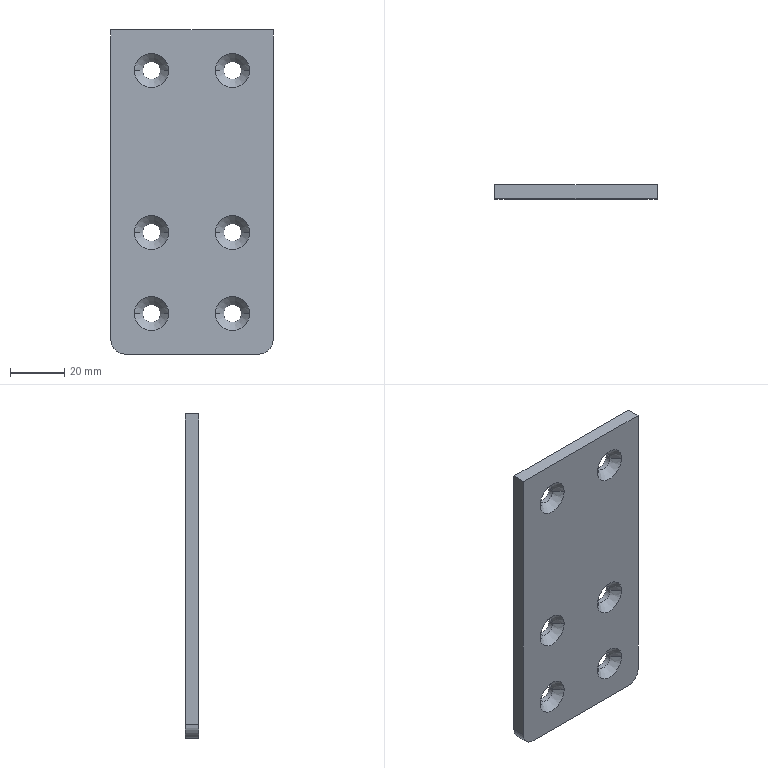Part | NX | features BREP 1 | 1 solid | 32 faces | box 60 x 5 x 120 mm | volume 34191 mm3 | cylinder 14 | cone 12 | plane 6 | commonest cylinder face diameters 6.6 x12 10 x2
STEP:
#1=CARTESIAN_POINT('',(-30.,0.,-70.));
#2=VERTEX_POINT('',#1);
#3=CARTESIAN_POINT('',(-30.,0.,45.));
#4=VERTEX_POINT('',#3);
#5=CARTESIAN_POINT('',(-30.,0.,-70.));
#6=DIRECTION('',(0.,0.,1.));
#7=VECTOR('',#6,1000.);
#8=LINE('',#5,#7);
#9=EDGE_CURVE('',#2,#4,#8,.T.);
#10=ORIENTED_EDGE('',*,*,#9,.F.);
#11=CARTESIAN_POINT('',(-25.,0.,-75.));
#12=VERTEX_POINT('',#11);
#13=CARTESIAN_POINT('',(-25.,0.,-70.));
#14=DIRECTION('',(0.,-1.,0.));
#15=DIRECTION('',(-1.,0.,0.));
#16=AXIS2_PLACEMENT_3D('',#13,#14,#15);
#17=CIRCLE('',#16,5.);
#18=EDGE_CURVE('',#2,#12,#17,.T.);
#19=ORIENTED_EDGE('',*,*,#18,.T.);
#20=CARTESIAN_POINT('',(25.,0.,-75.));
#21=VERTEX_POINT('',#20);
#22=CARTESIAN_POINT('',(25.,0.,-75.));
#23=DIRECTION('',(-1.,0.,0.));
#24=VECTOR('',#23,1000.);
#25=LINE('',#22,#24);
#26=EDGE_CURVE('',#21,#12,#25,.T.);
#27=ORIENTED_EDGE('',*,*,#26,.F.);
#28=CARTESIAN_POINT('',(30.,0.,-70.));
#29=VERTEX_POINT('',#28);
#30=CARTESIAN_POINT('',(25.,0.,-70.));
#31=DIRECTION('',(0.,-1.,0.));
#32=DIRECTION('',(0.,0.,-1.));
#33=AXIS2_PLACEMENT_3D('',#30,#31,#32);
#34=CIRCLE('',#33,5.);
#35=EDGE_CURVE('',#21,#29,#34,.T.);
#36=ORIENTED_EDGE('',*,*,#35,.T.);
#37=CARTESIAN_POINT('',(30.,0.,45.));
#38=VERTEX_POINT('',#37);
#39=CARTESIAN_POINT('',(30.,0.,45.));
#40=DIRECTION('',(0.,0.,-1.));
#41=VECTOR('',#40,1000.);
#42=LINE('',#39,#41);
#43=EDGE_CURVE('',#38,#29,#42,.T.);
#44=ORIENTED_EDGE('',*,*,#43,.F.);
#45=CARTESIAN_POINT('',(-30.,0.,45.));
#46=DIRECTION('',(1.,0.,0.));
#47=VECTOR('',#46,1000.);
#48=LINE('',#45,#47);
#49=EDGE_CURVE('',#4,#38,#48,.T.);
#50=ORIENTED_EDGE('',*,*,#49,.F.);
#51=EDGE_LOOP('',(#10,#19,#27,#36,#44,#50));
#52=FACE_BOUND('',#51,.T.);
#53=CARTESIAN_POINT('',(-8.7,0.,-60.));
#54=VERTEX_POINT('',#53);
#55=CARTESIAN_POINT('',(-21.3,0.,-60.));
#56=VERTEX_POINT('',#55);
#57=CARTESIAN_POINT('',(-15.,0.,-60.));
#58=DIRECTION('',(0.,-1.,0.));
#59=DIRECTION('',(1.,0.,0.));
#60=AXIS2_PLACEMENT_3D('',#57,#58,#59);
#61=CIRCLE('',#60,6.3);
#62=EDGE_CURVE('',#54,#56,#61,.T.);
#63=ORIENTED_EDGE('',*,*,#62,.F.);
#64=CARTESIAN_POINT('',(-15.,0.,-60.));
#65=DIRECTION('',(0.,-1.,0.));
#66=DIRECTION('',(-1.,0.,0.));
#67=AXIS2_PLACEMENT_3D('',#64,#65,#66);
#68=CIRCLE('',#67,6.3);
#69=EDGE_CURVE('',#56,#54,#68,.T.);
#70=ORIENTED_EDGE('',*,*,#69,.F.);
#71=EDGE_LOOP('',(#63,#70));
#72=FACE_BOUND('',#71,.T.);
#73=CARTESIAN_POINT('',(21.3,0.,-30.));
#74=VERTEX_POINT('',#73);
#75=CARTESIAN_POINT('',(8.7,0.,-30.));
#76=VERTEX_POINT('',#75);
#77=CARTESIAN_POINT('',(15.,0.,-30.));
#78=DIRECTION('',(0.,-1.,0.));
#79=DIRECTION('',(1.,0.,0.));
#80=AXIS2_PLACEMENT_3D('',#77,#78,#79);
#81=CIRCLE('',#80,6.3);
#82=EDGE_CURVE('',#74,#76,#81,.T.);
#83=ORIENTED_EDGE('',*,*,#82,.F.);
#84=CARTESIAN_POINT('',(15.,0.,-30.));
#85=DIRECTION('',(0.,-1.,0.));
#86=DIRECTION('',(-1.,0.,0.));
#87=AXIS2_PLACEMENT_3D('',#84,#85,#86);
#88=CIRCLE('',#87,6.3);
#89=EDGE_CURVE('',#76,#74,#88,.T.);
#90=ORIENTED_EDGE('',*,*,#89,.F.);
#91=EDGE_LOOP('',(#83,#90));
#92=FACE_BOUND('',#91,.T.);
#93=CARTESIAN_POINT('',(-8.7,0.,-30.));
#94=VERTEX_POINT('',#93);
#95=CARTESIAN_POINT('',(-21.3,0.,-30.));
#96=VERTEX_POINT('',#95);
#97=CARTESIAN_POINT('',(-15.,0.,-30.));
#98=DIRECTION('',(0.,-1.,0.));
#99=DIRECTION('',(1.,0.,0.));
#100=AXIS2_PLACEMENT_3D('',#97,#98,#99);
#101=CIRCLE('',#100,6.3);
#102=EDGE_CURVE('',#94,#96,#101,.T.);
#103=ORIENTED_EDGE('',*,*,#102,.F.);
#104=CARTESIAN_POINT('',(-15.,0.,-30.));
#105=DIRECTION('',(0.,-1.,0.));
#106=DIRECTION('',(-1.,0.,0.));
#107=AXIS2_PLACEMENT_3D('',#104,#105,#106);
#108=CIRCLE('',#107,6.3);
#109=EDGE_CURVE('',#96,#94,#108,.T.);
#110=ORIENTED_EDGE('',*,*,#109,.F.);
#111=EDGE_LOOP('',(#103,#110));
#112=FACE_BOUND('',#111,.T.);
#113=CARTESIAN_POINT('',(21.3,0.,30.));
#114=VERTEX_POINT('',#113);
#115=CARTESIAN_POINT('',(8.7,0.,30.));
#116=VERTEX_POINT('',#115);
#117=CARTESIAN_POINT('',(15.,0.,30.));
#118=DIRECTION('',(0.,1.,0.));
#119=DIRECTION('',(1.,0.,0.));
#120=AXIS2_PLACEMENT_3D('',#117,#118,#119);
#121=CIRCLE('',#120,6.3);
#122=EDGE_CURVE('',#114,#116,#121,.T.);
#123=ORIENTED_EDGE('',*,*,#122,.T.);
#124=CARTESIAN_POINT('',(15.,0.,30.));
#125=DIRECTION('',(0.,1.,0.));
#126=DIRECTION('',(-1.,0.,0.));
#127=AXIS2_PLACEMENT_3D('',#124,#125,#126);
#128=CIRCLE('',#127,6.3);
#129=EDGE_CURVE('',#116,#114,#128,.T.);
#130=ORIENTED_EDGE('',*,*,#129,.T.);
#131=EDGE_LOOP('',(#123,#130));
#132=FACE_BOUND('',#131,.T.);
#133=CARTESIAN_POINT('',(-8.7,0.,30.));
#134=VERTEX_POINT('',#133);
#135=CARTESIAN_POINT('',(-21.3,0.,30.));
#136=VERTEX_POINT('',#135);
#137=CARTESIAN_POINT('',(-15.,0.,30.));
#138=DIRECTION('',(0.,1.,0.));
#139=DIRECTION('',(1.,0.,0.));
#140=AXIS2_PLACEMENT_3D('',#137,#138,#139);
#141=CIRCLE('',#140,6.3);
#142=EDGE_CURVE('',#134,#136,#141,.T.);
#143=ORIENTED_EDGE('',*,*,#142,.T.);
#144=CARTESIAN_POINT('',(-15.,0.,30.));
#145=DIRECTION('',(0.,1.,0.));
#146=DIRECTION('',(-1.,0.,0.));
#147=AXIS2_PLACEMENT_3D('',#144,#145,#146);
#148=CIRCLE('',#147,6.3);
#149=EDGE_CURVE('',#136,#134,#148,.T.);
#150=ORIENTED_EDGE('',*,*,#149,.T.);
#151=EDGE_LOOP('',(#143,#150));
#152=FACE_BOUND('',#151,.T.);
#153=CARTESIAN_POINT('',(21.3,0.,-60.));
#154=VERTEX_POINT('',#153);
#155=CARTESIAN_POINT('',(8.7,0.,-60.));
#156=VERTEX_POINT('',#155);
#157=CARTESIAN_POINT('',(15.,0.,-60.));
#158=DIRECTION('',(0.,-1.,0.));
#159=DIRECTION('',(1.,0.,0.));
#160=AXIS2_PLACEMENT_3D('',#157,#158,#159);
#161=CIRCLE('',#160,6.3);
#162=EDGE_CURVE('',#154,#156,#161,.T.);
#163=ORIENTED_EDGE('',*,*,#162,.F.);
#164=CARTESIAN_POINT('',(15.,0.,-60.));
#165=DIRECTION('',(0.,-1.,0.));
#166=DIRECTION('',(-1.,0.,0.));
#167=AXIS2_PLACEMENT_3D('',#164,#165,#166);
#168=CIRCLE('',#167,6.3);
#169=EDGE_CURVE('',#156,#154,#168,.T.);
#170=ORIENTED_EDGE('',*,*,#169,.F.);
#171=EDGE_LOOP('',(#163,#170));
#172=FACE_BOUND('',#171,.T.);
#173=CARTESIAN_POINT('',(0.,0.,0.));
#174=DIRECTION('',(0.,1.,0.));
#175=DIRECTION('',(1.,0.,0.));
#176=AXIS2_PLACEMENT_3D('',#173,#174,#175);
#177=PLANE('',#176);
#178=ADVANCED_FACE('',(#52,#72,#92,#112,#132,#152,#172),#177,.F.);
#179=CARTESIAN_POINT('',(18.3,3.,-60.));
#180=VERTEX_POINT('',#179);
#181=CARTESIAN_POINT('',(18.3,3.,-60.));
#182=DIRECTION('',(0.7071,-0.7071,0.));
#183=VECTOR('',#182,1000.);
#184=LINE('',#181,#183);
#185=EDGE_CURVE('',#154,#180,#184,.F.);
#186=ORIENTED_EDGE('',*,*,#185,.T.);
#187=CARTESIAN_POINT('',(11.7,3.,-60.));
#188=VERTEX_POINT('',#187);
#189=CARTESIAN_POINT('',(15.,3.,-60.));
#190=DIRECTION('',(0.,-1.,0.));
#191=DIRECTION('',(-1.,0.,0.));
#192=AXIS2_PLACEMENT_3D('',#189,#190,#191);
#193=CIRCLE('',#192,3.3);
#194=EDGE_CURVE('',#188,#180,#193,.T.);
#195=ORIENTED_EDGE('',*,*,#194,.F.);
#196=CARTESIAN_POINT('',(11.7,3.,-60.));
#197=DIRECTION('',(-0.7071,-0.7071,0.));
#198=VECTOR('',#197,1000.);
#199=LINE('',#196,#198);
#200=EDGE_CURVE('',#156,#188,#199,.F.);
#201=ORIENTED_EDGE('',*,*,#200,.F.);
#202=ORIENTED_EDGE('',*,*,#169,.T.);
#203=EDGE_LOOP('',(#186,#195,#201,#202));
#204=FACE_BOUND('',#203,.T.);
#205=CARTESIAN_POINT('',(15.,1.5,-60.));
#206=DIRECTION('',(0.,-1.,0.));
#207=DIRECTION('',(-1.,0.,0.));
#208=AXIS2_PLACEMENT_3D('',#205,#206,#207);
#209=CONICAL_SURFACE('',#208,4.8,0.7854);
#210=ADVANCED_FACE('',(#204),#209,.F.);
#211=ORIENTED_EDGE('',*,*,#200,.T.);
#212=CARTESIAN_POINT('',(15.,3.,-60.));
#213=DIRECTION('',(0.,1.,0.));
#214=DIRECTION('',(-1.,0.,0.));
#215=AXIS2_PLACEMENT_3D('',#212,#213,#214);
#216=CIRCLE('',#215,3.3);
#217=EDGE_CURVE('',#188,#180,#216,.T.);
#218=ORIENTED_EDGE('',*,*,#217,.T.);
#219=ORIENTED_EDGE('',*,*,#185,.F.);
#220=ORIENTED_EDGE('',*,*,#162,.T.);
#221=EDGE_LOOP('',(#211,#218,#219,#220));
#222=FACE_BOUND('',#221,.T.);
#223=CARTESIAN_POINT('',(15.,1.5,-60.));
#224=DIRECTION('',(0.,-1.,0.));
#225=DIRECTION('',(-1.,0.,0.));
#226=AXIS2_PLACEMENT_3D('',#223,#224,#225);
#227=CONICAL_SURFACE('',#226,4.8,0.7854);
#228=ADVANCED_FACE('',(#222),#227,.F.);
#229=CARTESIAN_POINT('',(18.3,5.,-60.));
#230=VERTEX_POINT('',#229);
#231=CARTESIAN_POINT('',(18.3,5.,-60.));
#232=DIRECTION('',(0.,-1.,0.));
#233=VECTOR('',#232,1000.);
#234=LINE('',#231,#233);
#235=EDGE_CURVE('',#180,#230,#234,.F.);
#236=ORIENTED_EDGE('',*,*,#235,.F.);
#237=ORIENTED_EDGE('',*,*,#217,.F.);
#238=CARTESIAN_POINT('',(11.7,5.,-60.));
#239=VERTEX_POINT('',#238);
#240=CARTESIAN_POINT('',(11.7,5.,-60.));
#241=DIRECTION('',(0.,-1.,0.));
#242=VECTOR('',#241,1000.);
#243=LINE('',#240,#242);
#244=EDGE_CURVE('',#188,#239,#243,.F.);
#245=ORIENTED_EDGE('',*,*,#244,.T.);
#246=CARTESIAN_POINT('',(15.,5.,-60.));
#247=DIRECTION('',(0.,-1.,0.));
#248=DIRECTION('',(1.,0.,0.));
#249=AXIS2_PLACEMENT_3D('',#246,#247,#248);
#250=CIRCLE('',#249,3.3);
#251=EDGE_CURVE('',#230,#239,#250,.T.);
#252=ORIENTED_EDGE('',*,*,#251,.F.);
#253=EDGE_LOOP('',(#236,#237,#245,#252));
#254=FACE_BOUND('',#253,.T.);
#255=CARTESIAN_POINT('',(15.,44.512,-60.));
#256=DIRECTION('',(0.,-1.,0.));
#257=DIRECTION('',(-1.,0.,0.));
#258=AXIS2_PLACEMENT_3D('',#255,#256,#257);
#259=CYLINDRICAL_SURFACE('',#258,3.3);
#260=ADVANCED_FACE('',(#254),#259,.F.);
#261=CARTESIAN_POINT('',(30.,5.,45.));
#262=VERTEX_POINT('',#261);
#263=CARTESIAN_POINT('',(30.,5.,-70.));
#264=VERTEX_POINT('',#263);
#265=CARTESIAN_POINT('',(30.,5.,45.));
#266=DIRECTION('',(0.,0.,-1.));
#267=VECTOR('',#266,1000.);
#268=LINE('',#265,#267);
#269=EDGE_CURVE('',#262,#264,#268,.T.);
#270=ORIENTED_EDGE('',*,*,#269,.T.);
#271=CARTESIAN_POINT('',(25.,5.,-75.));
#272=VERTEX_POINT('',#271);
#273=CARTESIAN_POINT('',(25.,5.,-70.));
#274=DIRECTION('',(0.,1.,0.));
#275=DIRECTION('',(1.,0.,0.));
#276=AXIS2_PLACEMENT_3D('',#273,#274,#275);
#277=CIRCLE('',#276,5.);
#278=EDGE_CURVE('',#264,#272,#277,.T.);
#279=ORIENTED_EDGE('',*,*,#278,.T.);
#280=CARTESIAN_POINT('',(-25.,5.,-75.));
#281=VERTEX_POINT('',#280);
#282=CARTESIAN_POINT('',(25.,5.,-75.));
#283=DIRECTION('',(-1.,0.,0.));
#284=VECTOR('',#283,1000.);
#285=LINE('',#282,#284);
#286=EDGE_CURVE('',#272,#281,#285,.T.);
#287=ORIENTED_EDGE('',*,*,#286,.T.);
#288=CARTESIAN_POINT('',(-30.,5.,-70.));
#289=VERTEX_POINT('',#288);
#290=CARTESIAN_POINT('',(-25.,5.,-70.));
#291=DIRECTION('',(0.,1.,0.));
#292=DIRECTION('',(0.,0.,-1.));
#293=AXIS2_PLACEMENT_3D('',#290,#291,#292);
#294=CIRCLE('',#293,5.);
#295=EDGE_CURVE('',#281,#289,#294,.T.);
#296=ORIENTED_EDGE('',*,*,#295,.T.);
#297=CARTESIAN_POINT('',(-30.,5.,45.));
#298=VERTEX_POINT('',#297);
#299=CARTESIAN_POINT('',(-30.,5.,-70.));
#300=DIRECTION('',(0.,0.,1.));
#301=VECTOR('',#300,1000.);
#302=LINE('',#299,#301);
#303=EDGE_CURVE('',#289,#298,#302,.T.);
#304=ORIENTED_EDGE('',*,*,#303,.T.);
#305=CARTESIAN_POINT('',(-30.,5.,45.));
#306=DIRECTION('',(1.,0.,0.));
#307=VECTOR('',#306,1000.);
#308=LINE('',#305,#307);
#309=EDGE_CURVE('',#298,#262,#308,.T.);
#310=ORIENTED_EDGE('',*,*,#309,.T.);
#311=EDGE_LOOP('',(#270,#279,#287,#296,#304,#310));
#312=FACE_BOUND('',#311,.T.);
#313=CARTESIAN_POINT('',(-11.7,5.,-60.));
#314=VERTEX_POINT('',#313);
#315=CARTESIAN_POINT('',(-18.3,5.,-60.));
#316=VERTEX_POINT('',#315);
#317=CARTESIAN_POINT('',(-15.,5.,-60.));
#318=DIRECTION('',(0.,-1.,0.));
#319=DIRECTION('',(1.,0.,0.));
#320=AXIS2_PLACEMENT_3D('',#317,#318,#319);
#321=CIRCLE('',#320,3.3);
#322=EDGE_CURVE('',#314,#316,#321,.T.);
#323=ORIENTED_EDGE('',*,*,#322,.T.);
#324=CARTESIAN_POINT('',(-15.,5.,-60.));
#325=DIRECTION('',(0.,-1.,0.));
#326=DIRECTION('',(-1.,0.,0.));
#327=AXIS2_PLACEMENT_3D('',#324,#325,#326);
#328=CIRCLE('',#327,3.3);
#329=EDGE_CURVE('',#316,#314,#328,.T.);
#330=ORIENTED_EDGE('',*,*,#329,.T.);
#331=EDGE_LOOP('',(#323,#330));
#332=FACE_BOUND('',#331,.T.);
#333=CARTESIAN_POINT('',(18.3,5.,-30.));
#334=VERTEX_POINT('',#333);
#335=CARTESIAN_POINT('',(11.7,5.,-30.));
#336=VERTEX_POINT('',#335);
#337=CARTESIAN_POINT('',(15.,5.,-30.));
#338=DIRECTION('',(0.,-1.,0.));
#339=DIRECTION('',(1.,0.,0.));
#340=AXIS2_PLACEMENT_3D('',#337,#338,#339);
#341=CIRCLE('',#340,3.3);
#342=EDGE_CURVE('',#334,#336,#341,.T.);
#343=ORIENTED_EDGE('',*,*,#342,.T.);
#344=CARTESIAN_POINT('',(15.,5.,-30.));
#345=DIRECTION('',(0.,-1.,0.));
#346=DIRECTION('',(-1.,0.,0.));
#347=AXIS2_PLACEMENT_3D('',#344,#345,#346);
#348=CIRCLE('',#347,3.3);
#349=EDGE_CURVE('',#336,#334,#348,.T.);
#350=ORIENTED_EDGE('',*,*,#349,.T.);
#351=EDGE_LOOP('',(#343,#350));
#352=FACE_BOUND('',#351,.T.);
#353=CARTESIAN_POINT('',(-11.7,5.,-30.));
#354=VERTEX_POINT('',#353);
#355=CARTESIAN_POINT('',(-18.3,5.,-30.));
#356=VERTEX_POINT('',#355);
#357=CARTESIAN_POINT('',(-15.,5.,-30.));
#358=DIRECTION('',(0.,-1.,0.));
#359=DIRECTION('',(1.,0.,0.));
#360=AXIS2_PLACEMENT_3D('',#357,#358,#359);
#361=CIRCLE('',#360,3.3);
#362=EDGE_CURVE('',#354,#356,#361,.T.);
#363=ORIENTED_EDGE('',*,*,#362,.T.);
#364=CARTESIAN_POINT('',(-15.,5.,-30.));
#365=DIRECTION('',(0.,-1.,0.));
#366=DIRECTION('',(-1.,0.,0.));
#367=AXIS2_PLACEMENT_3D('',#364,#365,#366);
#368=CIRCLE('',#367,3.3);
#369=EDGE_CURVE('',#356,#354,#368,.T.);
#370=ORIENTED_EDGE('',*,*,#369,.T.);
#371=EDGE_LOOP('',(#363,#370));
#372=FACE_BOUND('',#371,.T.);
#373=CARTESIAN_POINT('',(18.3,5.,30.));
#374=VERTEX_POINT('',#373);
#375=CARTESIAN_POINT('',(11.7,5.,30.));
#376=VERTEX_POINT('',#375);
#377=CARTESIAN_POINT('',(15.,5.,30.));
#378=DIRECTION('',(0.,1.,0.));
#379=DIRECTION('',(1.,0.,0.));
#380=AXIS2_PLACEMENT_3D('',#377,#378,#379);
#381=CIRCLE('',#380,3.3);
#382=EDGE_CURVE('',#374,#376,#381,.T.);
#383=ORIENTED_EDGE('',*,*,#382,.F.);
#384=CARTESIAN_POINT('',(15.,5.,30.));
#385=DIRECTION('',(0.,1.,0.));
#386=DIRECTION('',(-1.,0.,0.));
#387=AXIS2_PLACEMENT_3D('',#384,#385,#386);
#388=CIRCLE('',#387,3.3);
#389=EDGE_CURVE('',#376,#374,#388,.T.);
#390=ORIENTED_EDGE('',*,*,#389,.F.);
#391=EDGE_LOOP('',(#383,#390));
#392=FACE_BOUND('',#391,.T.);
#393=CARTESIAN_POINT('',(-11.7,5.,30.));
#394=VERTEX_POINT('',#393);
#395=CARTESIAN_POINT('',(-18.3,5.,30.));
#396=VERTEX_POINT('',#395);
#397=CARTESIAN_POINT('',(-15.,5.,30.));
#398=DIRECTION('',(0.,1.,0.));
#399=DIRECTION('',(1.,0.,0.));
#400=AXIS2_PLACEMENT_3D('',#397,#398,#399);
#401=CIRCLE('',#400,3.3);
#402=EDGE_CURVE('',#394,#396,#401,.T.);
#403=ORIENTED_EDGE('',*,*,#402,.F.);
#404=CARTESIAN_POINT('',(-15.,5.,30.));
#405=DIRECTION('',(0.,1.,0.));
#406=DIRECTION('',(-1.,0.,0.));
#407=AXIS2_PLACEMENT_3D('',#404,#405,#406);
#408=CIRCLE('',#407,3.3);
#409=EDGE_CURVE('',#396,#394,#408,.T.);
#410=ORIENTED_EDGE('',*,*,#409,.F.);
#411=EDGE_LOOP('',(#403,#410));
#412=FACE_BOUND('',#411,.T.);
#413=ORIENTED_EDGE('',*,*,#251,.T.);
#414=CARTESIAN_POINT('',(15.,5.,-60.));
#415=DIRECTION('',(0.,-1.,0.));
#416=DIRECTION('',(-1.,0.,0.));
#417=AXIS2_PLACEMENT_3D('',#414,#415,#416);
#418=CIRCLE('',#417,3.3);
#419=EDGE_CURVE('',#239,#230,#418,.T.);
#420=ORIENTED_EDGE('',*,*,#419,.T.);
#421=EDGE_LOOP('',(#413,#420));
#422=FACE_BOUND('',#421,.T.);
#423=CARTESIAN_POINT('',(0.,5.,0.));
#424=DIRECTION('',(0.,1.,0.));
#425=DIRECTION('',(1.,0.,0.));
#426=AXIS2_PLACEMENT_3D('',#423,#424,#425);
#427=PLANE('',#426);
#428=ADVANCED_FACE('',(#312,#332,#352,#372,#392,#412,#422),#427,.T.);
#429=ORIENTED_EDGE('',*,*,#244,.F.);
#430=ORIENTED_EDGE('',*,*,#194,.T.);
#431=ORIENTED_EDGE('',*,*,#235,.T.);
#432=ORIENTED_EDGE('',*,*,#419,.F.);
#433=EDGE_LOOP('',(#429,#430,#431,#432));
#434=FACE_BOUND('',#433,.T.);
#435=CARTESIAN_POINT('',(15.,44.512,-60.));
#436=DIRECTION('',(0.,-1.,0.));
#437=DIRECTION('',(-1.,0.,0.));
#438=AXIS2_PLACEMENT_3D('',#435,#436,#437);
#439=CYLINDRICAL_SURFACE('',#438,3.3);
#440=ADVANCED_FACE('',(#434),#439,.F.);
#441=CARTESIAN_POINT('',(-18.3,3.,-60.));
#442=VERTEX_POINT('',#441);
#443=CARTESIAN_POINT('',(-18.3,5.,-60.));
#444=DIRECTION('',(0.,-1.,0.));
#445=VECTOR('',#444,1000.);
#446=LINE('',#443,#445);
#447=EDGE_CURVE('',#316,#442,#446,.T.);
#448=ORIENTED_EDGE('',*,*,#447,.T.);
#449=CARTESIAN_POINT('',(-11.7,3.,-60.));
#450=VERTEX_POINT('',#449);
#451=CARTESIAN_POINT('',(-15.,3.,-60.));
#452=DIRECTION('',(0.,-1.,0.));
#453=DIRECTION('',(-1.,0.,0.));
#454=AXIS2_PLACEMENT_3D('',#451,#452,#453);
#455=CIRCLE('',#454,3.3);
#456=EDGE_CURVE('',#442,#450,#455,.T.);
#457=ORIENTED_EDGE('',*,*,#456,.T.);
#458=CARTESIAN_POINT('',(-11.7,5.,-60.));
#459=DIRECTION('',(0.,-1.,0.));
#460=VECTOR('',#459,1000.);
#461=LINE('',#458,#460);
#462=EDGE_CURVE('',#314,#450,#461,.T.);
#463=ORIENTED_EDGE('',*,*,#462,.F.);
#464=ORIENTED_EDGE('',*,*,#329,.F.);
#465=EDGE_LOOP('',(#448,#457,#463,#464));
#466=FACE_BOUND('',#465,.T.);
#467=CARTESIAN_POINT('',(-15.,44.512,-60.));
#468=DIRECTION('',(0.,-1.,0.));
#469=DIRECTION('',(-1.,0.,0.));
#470=AXIS2_PLACEMENT_3D('',#467,#468,#469);
#471=CYLINDRICAL_SURFACE('',#470,3.3);
#472=ADVANCED_FACE('',(#466),#471,.F.);
#473=ORIENTED_EDGE('',*,*,#462,.T.);
#474=CARTESIAN_POINT('',(-15.,3.,-60.));
#475=DIRECTION('',(0.,1.,0.));
#476=DIRECTION('',(-1.,0.,0.));
#477=AXIS2_PLACEMENT_3D('',#474,#475,#476);
#478=CIRCLE('',#477,3.3);
#479=EDGE_CURVE('',#442,#450,#478,.T.);
#480=ORIENTED_EDGE('',*,*,#479,.F.);
#481=ORIENTED_EDGE('',*,*,#447,.F.);
#482=ORIENTED_EDGE('',*,*,#322,.F.);
#483=EDGE_LOOP('',(#473,#480,#481,#482));
#484=FACE_BOUND('',#483,.T.);
#485=CARTESIAN_POINT('',(-15.,44.512,-60.));
#486=DIRECTION('',(0.,-1.,0.));
#487=DIRECTION('',(-1.,0.,0.));
#488=AXIS2_PLACEMENT_3D('',#485,#486,#487);
#489=CYLINDRICAL_SURFACE('',#488,3.3);
#490=ADVANCED_FACE('',(#484),#489,.F.);
#491=CARTESIAN_POINT('',(-18.3,3.,-60.));
#492=DIRECTION('',(-0.7071,-0.7071,0.));
#493=VECTOR('',#492,1000.);
#494=LINE('',#491,#493);
#495=EDGE_CURVE('',#442,#56,#494,.T.);
#496=ORIENTED_EDGE('',*,*,#495,.F.);
#497=ORIENTED_EDGE('',*,*,#479,.T.);
#498=CARTESIAN_POINT('',(-11.7,3.,-60.));
#499=DIRECTION('',(0.7071,-0.7071,0.));
#500=VECTOR('',#499,1000.);
#501=LINE('',#498,#500);
#502=EDGE_CURVE('',#450,#54,#501,.T.);
#503=ORIENTED_EDGE('',*,*,#502,.T.);
#504=ORIENTED_EDGE('',*,*,#62,.T.);
#505=EDGE_LOOP('',(#496,#497,#503,#504));
#506=FACE_BOUND('',#505,.T.);
#507=CARTESIAN_POINT('',(-15.,1.5,-60.));
#508=DIRECTION('',(0.,-1.,0.));
#509=DIRECTION('',(-1.,0.,0.));
#510=AXIS2_PLACEMENT_3D('',#507,#508,#509);
#511=CONICAL_SURFACE('',#510,4.8,0.7854);
#512=ADVANCED_FACE('',(#506),#511,.F.);
#513=ORIENTED_EDGE('',*,*,#502,.F.);
#514=ORIENTED_EDGE('',*,*,#456,.F.);
#515=ORIENTED_EDGE('',*,*,#495,.T.);
#516=ORIENTED_EDGE('',*,*,#69,.T.);
#517=EDGE_LOOP('',(#513,#514,#515,#516));
#518=FACE_BOUND('',#517,.T.);
#519=CARTESIAN_POINT('',(-15.,1.5,-60.));
#520=DIRECTION('',(0.,-1.,0.));
#521=DIRECTION('',(-1.,0.,0.));
#522=AXIS2_PLACEMENT_3D('',#519,#520,#521);
#523=CONICAL_SURFACE('',#522,4.8,0.7854);
#524=ADVANCED_FACE('',(#518),#523,.F.);
#525=CARTESIAN_POINT('',(11.7,3.,-30.));
#526=VERTEX_POINT('',#525);
#527=CARTESIAN_POINT('',(11.7,5.,-30.));
#528=DIRECTION('',(0.,-1.,0.));
#529=VECTOR('',#528,1000.);
#530=LINE('',#527,#529);
#531=EDGE_CURVE('',#336,#526,#530,.T.);
#532=ORIENTED_EDGE('',*,*,#531,.T.);
#533=CARTESIAN_POINT('',(18.3,3.,-30.));
#534=VERTEX_POINT('',#533);
#535=CARTESIAN_POINT('',(15.,3.,-30.));
#536=DIRECTION('',(0.,-1.,0.));
#537=DIRECTION('',(-1.,0.,0.));
#538=AXIS2_PLACEMENT_3D('',#535,#536,#537);
#539=CIRCLE('',#538,3.3);
#540=EDGE_CURVE('',#526,#534,#539,.T.);
#541=ORIENTED_EDGE('',*,*,#540,.T.);
#542=CARTESIAN_POINT('',(18.3,5.,-30.));
#543=DIRECTION('',(0.,-1.,0.));
#544=VECTOR('',#543,1000.);
#545=LINE('',#542,#544);
#546=EDGE_CURVE('',#334,#534,#545,.T.);
#547=ORIENTED_EDGE('',*,*,#546,.F.);
#548=ORIENTED_EDGE('',*,*,#349,.F.);
#549=EDGE_LOOP('',(#532,#541,#547,#548));
#550=FACE_BOUND('',#549,.T.);
#551=CARTESIAN_POINT('',(15.,44.512,-30.));
#552=DIRECTION('',(0.,-1.,0.));
#553=DIRECTION('',(-1.,0.,0.));
#554=AXIS2_PLACEMENT_3D('',#551,#552,#553);
#555=CYLINDRICAL_SURFACE('',#554,3.3);
#556=ADVANCED_FACE('',(#550),#555,.F.);
#557=ORIENTED_EDGE('',*,*,#546,.T.);
#558=CARTESIAN_POINT('',(15.,3.,-30.));
#559=DIRECTION('',(0.,1.,0.));
#560=DIRECTION('',(-1.,0.,0.));
#561=AXIS2_PLACEMENT_3D('',#558,#559,#560);
#562=CIRCLE('',#561,3.3);
#563=EDGE_CURVE('',#526,#534,#562,.T.);
#564=ORIENTED_EDGE('',*,*,#563,.F.);
#565=ORIENTED_EDGE('',*,*,#531,.F.);
#566=ORIENTED_EDGE('',*,*,#342,.F.);
#567=EDGE_LOOP('',(#557,#564,#565,#566));
#568=FACE_BOUND('',#567,.T.);
#569=CARTESIAN_POINT('',(15.,44.512,-30.));
#570=DIRECTION('',(0.,-1.,0.));
#571=DIRECTION('',(-1.,0.,0.));
#572=AXIS2_PLACEMENT_3D('',#569,#570,#571);
#573=CYLINDRICAL_SURFACE('',#572,3.3);
#574=ADVANCED_FACE('',(#568),#573,.F.);
#575=CARTESIAN_POINT('',(11.7,3.,-30.));
#576=DIRECTION('',(-0.7071,-0.7071,0.));
#577=VECTOR('',#576,1000.);
#578=LINE('',#575,#577);
#579=EDGE_CURVE('',#526,#76,#578,.T.);
#580=ORIENTED_EDGE('',*,*,#579,.F.);
#581=ORIENTED_EDGE('',*,*,#563,.T.);
#582=CARTESIAN_POINT('',(18.3,3.,-30.));
#583=DIRECTION('',(0.7071,-0.7071,0.));
#584=VECTOR('',#583,1000.);
#585=LINE('',#582,#584);
#586=EDGE_CURVE('',#534,#74,#585,.T.);
#587=ORIENTED_EDGE('',*,*,#586,.T.);
#588=ORIENTED_EDGE('',*,*,#82,.T.);
#589=EDGE_LOOP('',(#580,#581,#587,#588));
#590=FACE_BOUND('',#589,.T.);
#591=CARTESIAN_POINT('',(15.,1.5,-30.));
#592=DIRECTION('',(0.,-1.,0.));
#593=DIRECTION('',(-1.,0.,0.));
#594=AXIS2_PLACEMENT_3D('',#591,#592,#593);
#595=CONICAL_SURFACE('',#594,4.8,0.7854);
#596=ADVANCED_FACE('',(#590),#595,.F.);
#597=ORIENTED_EDGE('',*,*,#586,.F.);
#598=ORIENTED_EDGE('',*,*,#540,.F.);
#599=ORIENTED_EDGE('',*,*,#579,.T.);
#600=ORIENTED_EDGE('',*,*,#89,.T.);
#601=EDGE_LOOP('',(#597,#598,#599,#600));
#602=FACE_BOUND('',#601,.T.);
#603=CARTESIAN_POINT('',(15.,1.5,-30.));
#604=DIRECTION('',(0.,-1.,0.));
#605=DIRECTION('',(-1.,0.,0.));
#606=AXIS2_PLACEMENT_3D('',#603,#604,#605);
#607=CONICAL_SURFACE('',#606,4.8,0.7854);
#608=ADVANCED_FACE('',(#602),#607,.F.);
#609=CARTESIAN_POINT('',(-18.3,3.,-30.));
#610=VERTEX_POINT('',#609);
#611=CARTESIAN_POINT('',(-18.3,5.,-30.));
#612=DIRECTION('',(0.,-1.,0.));
#613=VECTOR('',#612,1000.);
#614=LINE('',#611,#613);
#615=EDGE_CURVE('',#356,#610,#614,.T.);
#616=ORIENTED_EDGE('',*,*,#615,.T.);
#617=CARTESIAN_POINT('',(-11.7,3.,-30.));
#618=VERTEX_POINT('',#617);
#619=CARTESIAN_POINT('',(-15.,3.,-30.));
#620=DIRECTION('',(0.,-1.,0.));
#621=DIRECTION('',(-1.,0.,0.));
#622=AXIS2_PLACEMENT_3D('',#619,#620,#621);
#623=CIRCLE('',#622,3.3);
#624=EDGE_CURVE('',#610,#618,#623,.T.);
#625=ORIENTED_EDGE('',*,*,#624,.T.);
#626=CARTESIAN_POINT('',(-11.7,5.,-30.));
#627=DIRECTION('',(0.,-1.,0.));
#628=VECTOR('',#627,1000.);
#629=LINE('',#626,#628);
#630=EDGE_CURVE('',#354,#618,#629,.T.);
#631=ORIENTED_EDGE('',*,*,#630,.F.);
#632=ORIENTED_EDGE('',*,*,#369,.F.);
#633=EDGE_LOOP('',(#616,#625,#631,#632));
#634=FACE_BOUND('',#633,.T.);
#635=CARTESIAN_POINT('',(-15.,44.512,-30.));
#636=DIRECTION('',(0.,-1.,0.));
#637=DIRECTION('',(-1.,0.,0.));
#638=AXIS2_PLACEMENT_3D('',#635,#636,#637);
#639=CYLINDRICAL_SURFACE('',#638,3.3);
#640=ADVANCED_FACE('',(#634),#639,.F.);
#641=ORIENTED_EDGE('',*,*,#630,.T.);
#642=CARTESIAN_POINT('',(-15.,3.,-30.));
#643=DIRECTION('',(0.,1.,0.));
#644=DIRECTION('',(-1.,0.,0.));
#645=AXIS2_PLACEMENT_3D('',#642,#643,#644);
#646=CIRCLE('',#645,3.3);
#647=EDGE_CURVE('',#610,#618,#646,.T.);
#648=ORIENTED_EDGE('',*,*,#647,.F.);
#649=ORIENTED_EDGE('',*,*,#615,.F.);
#650=ORIENTED_EDGE('',*,*,#362,.F.);
#651=EDGE_LOOP('',(#641,#648,#649,#650));
#652=FACE_BOUND('',#651,.T.);
#653=CARTESIAN_POINT('',(-15.,44.512,-30.));
#654=DIRECTION('',(0.,-1.,0.));
#655=DIRECTION('',(-1.,0.,0.));
#656=AXIS2_PLACEMENT_3D('',#653,#654,#655);
#657=CYLINDRICAL_SURFACE('',#656,3.3);
#658=ADVANCED_FACE('',(#652),#657,.F.);
#659=CARTESIAN_POINT('',(-18.3,3.,-30.));
#660=DIRECTION('',(-0.7071,-0.7071,0.));
#661=VECTOR('',#660,1000.);
#662=LINE('',#659,#661);
#663=EDGE_CURVE('',#610,#96,#662,.T.);
#664=ORIENTED_EDGE('',*,*,#663,.F.);
#665=ORIENTED_EDGE('',*,*,#647,.T.);
#666=CARTESIAN_POINT('',(-11.7,3.,-30.));
#667=DIRECTION('',(0.7071,-0.7071,0.));
#668=VECTOR('',#667,1000.);
#669=LINE('',#666,#668);
#670=EDGE_CURVE('',#618,#94,#669,.T.);
#671=ORIENTED_EDGE('',*,*,#670,.T.);
#672=ORIENTED_EDGE('',*,*,#102,.T.);
#673=EDGE_LOOP('',(#664,#665,#671,#672));
#674=FACE_BOUND('',#673,.T.);
#675=CARTESIAN_POINT('',(-15.,1.5,-30.));
#676=DIRECTION('',(0.,-1.,0.));
#677=DIRECTION('',(-1.,0.,0.));
#678=AXIS2_PLACEMENT_3D('',#675,#676,#677);
#679=CONICAL_SURFACE('',#678,4.8,0.7854);
#680=ADVANCED_FACE('',(#674),#679,.F.);
#681=ORIENTED_EDGE('',*,*,#670,.F.);
#682=ORIENTED_EDGE('',*,*,#624,.F.);
#683=ORIENTED_EDGE('',*,*,#663,.T.);
#684=ORIENTED_EDGE('',*,*,#109,.T.);
#685=EDGE_LOOP('',(#681,#682,#683,#684));
#686=FACE_BOUND('',#685,.T.);
#687=CARTESIAN_POINT('',(-15.,1.5,-30.));
#688=DIRECTION('',(0.,-1.,0.));
#689=DIRECTION('',(-1.,0.,0.));
#690=AXIS2_PLACEMENT_3D('',#687,#688,#689);
#691=CONICAL_SURFACE('',#690,4.8,0.7854);
#692=ADVANCED_FACE('',(#686),#691,.F.);
#693=ORIENTED_EDGE('',*,*,#389,.T.);
#694=CARTESIAN_POINT('',(18.3,3.,30.));
#695=VERTEX_POINT('',#694);
#696=CARTESIAN_POINT('',(18.3,5.,30.));
#697=DIRECTION('',(0.,-1.,0.));
#698=VECTOR('',#697,1000.);
#699=LINE('',#696,#698);
#700=EDGE_CURVE('',#374,#695,#699,.T.);
#701=ORIENTED_EDGE('',*,*,#700,.T.);
#702=CARTESIAN_POINT('',(11.7,3.,30.));
#703=VERTEX_POINT('',#702);
#704=CARTESIAN_POINT('',(15.,3.,30.));
#705=DIRECTION('',(0.,1.,0.));
#706=DIRECTION('',(-1.,0.,0.));
#707=AXIS2_PLACEMENT_3D('',#704,#705,#706);
#708=CIRCLE('',#707,3.3);
#709=EDGE_CURVE('',#703,#695,#708,.T.);
#710=ORIENTED_EDGE('',*,*,#709,.F.);
#711=CARTESIAN_POINT('',(11.7,5.,30.));
#712=DIRECTION('',(0.,-1.,0.));
#713=VECTOR('',#712,1000.);
#714=LINE('',#711,#713);
#715=EDGE_CURVE('',#376,#703,#714,.T.);
#716=ORIENTED_EDGE('',*,*,#715,.F.);
#717=EDGE_LOOP('',(#693,#701,#710,#716));
#718=FACE_BOUND('',#717,.T.);
#719=CARTESIAN_POINT('',(15.,44.512,30.));
#720=DIRECTION('',(0.,1.,0.));
#721=DIRECTION('',(-1.,0.,0.));
#722=AXIS2_PLACEMENT_3D('',#719,#720,#721);
#723=CYLINDRICAL_SURFACE('',#722,3.3);
#724=ADVANCED_FACE('',(#718),#723,.F.);
#725=CARTESIAN_POINT('',(15.,3.,30.));
#726=DIRECTION('',(0.,-1.,0.));
#727=DIRECTION('',(-1.,0.,0.));
#728=AXIS2_PLACEMENT_3D('',#725,#726,#727);
#729=CIRCLE('',#728,3.3);
#730=EDGE_CURVE('',#703,#695,#729,.T.);
#731=ORIENTED_EDGE('',*,*,#730,.T.);
#732=ORIENTED_EDGE('',*,*,#700,.F.);
#733=ORIENTED_EDGE('',*,*,#382,.T.);
#734=ORIENTED_EDGE('',*,*,#715,.T.);
#735=EDGE_LOOP('',(#731,#732,#733,#734));
#736=FACE_BOUND('',#735,.T.);
#737=CARTESIAN_POINT('',(15.,44.512,30.));
#738=DIRECTION('',(0.,1.,0.));
#739=DIRECTION('',(-1.,0.,0.));
#740=AXIS2_PLACEMENT_3D('',#737,#738,#739);
#741=CYLINDRICAL_SURFACE('',#740,3.3);
#742=ADVANCED_FACE('',(#736),#741,.F.);
#743=ORIENTED_EDGE('',*,*,#122,.F.);
#744=CARTESIAN_POINT('',(18.3,3.,30.));
#745=DIRECTION('',(0.7071,-0.7071,0.));
#746=VECTOR('',#745,1000.);
#747=LINE('',#744,#746);
#748=EDGE_CURVE('',#695,#114,#747,.T.);
#749=ORIENTED_EDGE('',*,*,#748,.F.);
#750=ORIENTED_EDGE('',*,*,#730,.F.);
#751=CARTESIAN_POINT('',(11.7,3.,30.));
#752=DIRECTION('',(-0.7071,-0.7071,0.));
#753=VECTOR('',#752,1000.);
#754=LINE('',#751,#753);
#755=EDGE_CURVE('',#703,#116,#754,.T.);
#756=ORIENTED_EDGE('',*,*,#755,.T.);
#757=EDGE_LOOP('',(#743,#749,#750,#756));
#758=FACE_BOUND('',#757,.T.);
#759=CARTESIAN_POINT('',(15.,1.5,30.));
#760=DIRECTION('',(0.,-1.,0.));
#761=DIRECTION('',(1.,0.,0.));
#762=AXIS2_PLACEMENT_3D('',#759,#760,#761);
#763=CONICAL_SURFACE('',#762,4.8,0.7854);
#764=ADVANCED_FACE('',(#758),#763,.F.);
#765=ORIENTED_EDGE('',*,*,#709,.T.);
#766=ORIENTED_EDGE('',*,*,#748,.T.);
#767=ORIENTED_EDGE('',*,*,#129,.F.);
#768=ORIENTED_EDGE('',*,*,#755,.F.);
#769=EDGE_LOOP('',(#765,#766,#767,#768));
#770=FACE_BOUND('',#769,.T.);
#771=CARTESIAN_POINT('',(15.,1.5,30.));
#772=DIRECTION('',(0.,-1.,0.));
#773=DIRECTION('',(1.,0.,0.));
#774=AXIS2_PLACEMENT_3D('',#771,#772,#773);
#775=CONICAL_SURFACE('',#774,4.8,0.7854);
#776=ADVANCED_FACE('',(#770),#775,.F.);
#777=ORIENTED_EDGE('',*,*,#409,.T.);
#778=CARTESIAN_POINT('',(-11.7,3.,30.));
#779=VERTEX_POINT('',#778);
#780=CARTESIAN_POINT('',(-11.7,5.,30.));
#781=DIRECTION('',(0.,-1.,0.));
#782=VECTOR('',#781,1000.);
#783=LINE('',#780,#782);
#784=EDGE_CURVE('',#394,#779,#783,.T.);
#785=ORIENTED_EDGE('',*,*,#784,.T.);
#786=CARTESIAN_POINT('',(-18.3,3.,30.));
#787=VERTEX_POINT('',#786);
#788=CARTESIAN_POINT('',(-15.,3.,30.));
#789=DIRECTION('',(0.,1.,0.));
#790=DIRECTION('',(-1.,0.,0.));
#791=AXIS2_PLACEMENT_3D('',#788,#789,#790);
#792=CIRCLE('',#791,3.3);
#793=EDGE_CURVE('',#787,#779,#792,.T.);
#794=ORIENTED_EDGE('',*,*,#793,.F.);
#795=CARTESIAN_POINT('',(-18.3,5.,30.));
#796=DIRECTION('',(0.,-1.,0.));
#797=VECTOR('',#796,1000.);
#798=LINE('',#795,#797);
#799=EDGE_CURVE('',#396,#787,#798,.T.);
#800=ORIENTED_EDGE('',*,*,#799,.F.);
#801=EDGE_LOOP('',(#777,#785,#794,#800));
#802=FACE_BOUND('',#801,.T.);
#803=CARTESIAN_POINT('',(-15.,44.512,30.));
#804=DIRECTION('',(0.,1.,0.));
#805=DIRECTION('',(-1.,0.,0.));
#806=AXIS2_PLACEMENT_3D('',#803,#804,#805);
#807=CYLINDRICAL_SURFACE('',#806,3.3);
#808=ADVANCED_FACE('',(#802),#807,.F.);
#809=CARTESIAN_POINT('',(-15.,3.,30.));
#810=DIRECTION('',(0.,-1.,0.));
#811=DIRECTION('',(-1.,0.,0.));
#812=AXIS2_PLACEMENT_3D('',#809,#810,#811);
#813=CIRCLE('',#812,3.3);
#814=EDGE_CURVE('',#787,#779,#813,.T.);
#815=ORIENTED_EDGE('',*,*,#814,.T.);
#816=ORIENTED_EDGE('',*,*,#784,.F.);
#817=ORIENTED_EDGE('',*,*,#402,.T.);
#818=ORIENTED_EDGE('',*,*,#799,.T.);
#819=EDGE_LOOP('',(#815,#816,#817,#818));
#820=FACE_BOUND('',#819,.T.);
#821=CARTESIAN_POINT('',(-15.,44.512,30.));
#822=DIRECTION('',(0.,1.,0.));
#823=DIRECTION('',(-1.,0.,0.));
#824=AXIS2_PLACEMENT_3D('',#821,#822,#823);
#825=CYLINDRICAL_SURFACE('',#824,3.3);
#826=ADVANCED_FACE('',(#820),#825,.F.);
#827=ORIENTED_EDGE('',*,*,#142,.F.);
#828=CARTESIAN_POINT('',(-11.7,3.,30.));
#829=DIRECTION('',(0.7071,-0.7071,0.));
#830=VECTOR('',#829,1000.);
#831=LINE('',#828,#830);
#832=EDGE_CURVE('',#779,#134,#831,.T.);
#833=ORIENTED_EDGE('',*,*,#832,.F.);
#834=ORIENTED_EDGE('',*,*,#814,.F.);
#835=CARTESIAN_POINT('',(-18.3,3.,30.));
#836=DIRECTION('',(-0.7071,-0.7071,0.));
#837=VECTOR('',#836,1000.);
#838=LINE('',#835,#837);
#839=EDGE_CURVE('',#787,#136,#838,.T.);
#840=ORIENTED_EDGE('',*,*,#839,.T.);
#841=EDGE_LOOP('',(#827,#833,#834,#840));
#842=FACE_BOUND('',#841,.T.);
#843=CARTESIAN_POINT('',(-15.,1.5,30.));
#844=DIRECTION('',(0.,-1.,0.));
#845=DIRECTION('',(1.,0.,0.));
#846=AXIS2_PLACEMENT_3D('',#843,#844,#845);
#847=CONICAL_SURFACE('',#846,4.8,0.7854);
#848=ADVANCED_FACE('',(#842),#847,.F.);
#849=ORIENTED_EDGE('',*,*,#793,.T.);
#850=ORIENTED_EDGE('',*,*,#832,.T.);
#851=ORIENTED_EDGE('',*,*,#149,.F.);
#852=ORIENTED_EDGE('',*,*,#839,.F.);
#853=EDGE_LOOP('',(#849,#850,#851,#852));
#854=FACE_BOUND('',#853,.T.);
#855=CARTESIAN_POINT('',(-15.,1.5,30.));
#856=DIRECTION('',(0.,-1.,0.));
#857=DIRECTION('',(1.,0.,0.));
#858=AXIS2_PLACEMENT_3D('',#855,#856,#857);
#859=CONICAL_SURFACE('',#858,4.8,0.7854);
#860=ADVANCED_FACE('',(#854),#859,.F.);
#861=CARTESIAN_POINT('',(30.,0.,45.));
#862=DIRECTION('',(0.,1.,0.));
#863=VECTOR('',#862,1000.);
#864=LINE('',#861,#863);
#865=EDGE_CURVE('',#38,#262,#864,.T.);
#866=ORIENTED_EDGE('',*,*,#865,.T.);
#867=ORIENTED_EDGE('',*,*,#309,.F.);
#868=CARTESIAN_POINT('',(-30.,0.,45.));
#869=DIRECTION('',(0.,1.,0.));
#870=VECTOR('',#869,1000.);
#871=LINE('',#868,#870);
#872=EDGE_CURVE('',#4,#298,#871,.T.);
#873=ORIENTED_EDGE('',*,*,#872,.F.);
#874=ORIENTED_EDGE('',*,*,#49,.T.);
#875=EDGE_LOOP('',(#866,#867,#873,#874));
#876=FACE_BOUND('',#875,.T.);
#877=CARTESIAN_POINT('',(-30.,0.,45.));
#878=DIRECTION('',(0.,0.,-1.));
#879=DIRECTION('',(0.,-1.,0.));
#880=AXIS2_PLACEMENT_3D('',#877,#878,#879);
#881=PLANE('',#880);
#882=ADVANCED_FACE('',(#876),#881,.F.);
#883=ORIENTED_EDGE('',*,*,#303,.F.);
#884=CARTESIAN_POINT('',(-30.,5.,-70.));
#885=DIRECTION('',(0.,-1.,0.));
#886=VECTOR('',#885,1000.);
#887=LINE('',#884,#886);
#888=EDGE_CURVE('',#289,#2,#887,.T.);
#889=ORIENTED_EDGE('',*,*,#888,.T.);
#890=ORIENTED_EDGE('',*,*,#9,.T.);
#891=ORIENTED_EDGE('',*,*,#872,.T.);
#892=EDGE_LOOP('',(#883,#889,#890,#891));
#893=FACE_BOUND('',#892,.T.);
#894=CARTESIAN_POINT('',(-30.,0.,-75.));
#895=DIRECTION('',(-1.,0.,0.));
#896=DIRECTION('',(0.,0.,1.));
#897=AXIS2_PLACEMENT_3D('',#894,#895,#896);
#898=PLANE('',#897);
#899=ADVANCED_FACE('',(#893),#898,.T.);
#900=ORIENTED_EDGE('',*,*,#888,.F.);
#901=ORIENTED_EDGE('',*,*,#295,.F.);
#902=CARTESIAN_POINT('',(-25.,5.,-75.));
#903=DIRECTION('',(0.,-1.,0.));
#904=VECTOR('',#903,1000.);
#905=LINE('',#902,#904);
#906=EDGE_CURVE('',#281,#12,#905,.T.);
#907=ORIENTED_EDGE('',*,*,#906,.T.);
#908=ORIENTED_EDGE('',*,*,#18,.F.);
#909=EDGE_LOOP('',(#900,#901,#907,#908));
#910=FACE_BOUND('',#909,.T.);
#911=CARTESIAN_POINT('',(-25.,11.518,-70.));
#912=DIRECTION('',(0.,-1.,0.));
#913=DIRECTION('',(-1.,0.,0.));
#914=AXIS2_PLACEMENT_3D('',#911,#912,#913);
#915=CYLINDRICAL_SURFACE('',#914,5.);
#916=ADVANCED_FACE('',(#910),#915,.T.);
#917=ORIENTED_EDGE('',*,*,#26,.T.);
#918=ORIENTED_EDGE('',*,*,#906,.F.);
#919=ORIENTED_EDGE('',*,*,#286,.F.);
#920=CARTESIAN_POINT('',(25.,5.,-75.));
#921=DIRECTION('',(0.,-1.,0.));
#922=VECTOR('',#921,1000.);
#923=LINE('',#920,#922);
#924=EDGE_CURVE('',#272,#21,#923,.T.);
#925=ORIENTED_EDGE('',*,*,#924,.T.);
#926=EDGE_LOOP('',(#917,#918,#919,#925));
#927=FACE_BOUND('',#926,.T.);
#928=CARTESIAN_POINT('',(30.,0.,-75.));
#929=DIRECTION('',(0.,0.,-1.));
#930=DIRECTION('',(0.,-1.,0.));
#931=AXIS2_PLACEMENT_3D('',#928,#929,#930);
#932=PLANE('',#931);
#933=ADVANCED_FACE('',(#927),#932,.T.);
#934=ORIENTED_EDGE('',*,*,#924,.F.);
#935=ORIENTED_EDGE('',*,*,#278,.F.);
#936=CARTESIAN_POINT('',(30.,5.,-70.));
#937=DIRECTION('',(0.,-1.,0.));
#938=VECTOR('',#937,1000.);
#939=LINE('',#936,#938);
#940=EDGE_CURVE('',#264,#29,#939,.T.);
#941=ORIENTED_EDGE('',*,*,#940,.T.);
#942=ORIENTED_EDGE('',*,*,#35,.F.);
#943=EDGE_LOOP('',(#934,#935,#941,#942));
#944=FACE_BOUND('',#943,.T.);
#945=CARTESIAN_POINT('',(25.,11.518,-70.));
#946=DIRECTION('',(0.,-1.,0.));
#947=DIRECTION('',(0.,0.,-1.));
#948=AXIS2_PLACEMENT_3D('',#945,#946,#947);
#949=CYLINDRICAL_SURFACE('',#948,5.);
#950=ADVANCED_FACE('',(#944),#949,.T.);
#951=ORIENTED_EDGE('',*,*,#43,.T.);
#952=ORIENTED_EDGE('',*,*,#940,.F.);
#953=ORIENTED_EDGE('',*,*,#269,.F.);
#954=ORIENTED_EDGE('',*,*,#865,.F.);
#955=EDGE_LOOP('',(#951,#952,#953,#954));
#956=FACE_BOUND('',#955,.T.);
#957=CARTESIAN_POINT('',(30.,0.,75.));
#958=DIRECTION('',(1.,0.,0.));
#959=DIRECTION('',(0.,1.,0.));
#960=AXIS2_PLACEMENT_3D('',#957,#958,#959);
#961=PLANE('',#960);
#962=ADVANCED_FACE('',(#956),#961,.T.);
#963=CLOSED_SHELL('',(#178,#210,#228,#260,#428,#440,#472,#490,#512,#524,#556,#574,#596,#608,#640,#658,#680,#692,#724,#742,#764,#776,#808,#826,#848,#860,#882,#899,#916,#933,#950,#962));
#964=MANIFOLD_SOLID_BREP('',#963);
#965=(LENGTH_UNIT()NAMED_UNIT(*)SI_UNIT(.MILLI.,.METRE.));
#966=UNCERTAINTY_MEASURE_WITH_UNIT(LENGTH_MEASURE(0.00001),#965,'','');
#967=(NAMED_UNIT(*)PLANE_ANGLE_UNIT()SI_UNIT($,.RADIAN.));
#968=(NAMED_UNIT(*)SI_UNIT($,.STERADIAN.)SOLID_ANGLE_UNIT());
#969=(GEOMETRIC_REPRESENTATION_CONTEXT(3)GLOBAL_UNCERTAINTY_ASSIGNED_CONTEXT((#966))GLOBAL_UNIT_ASSIGNED_CONTEXT((#965,#967,#968))REPRESENTATION_CONTEXT('',''));
#970=ADVANCED_BREP_SHAPE_REPRESENTATION('',(#964),#969);